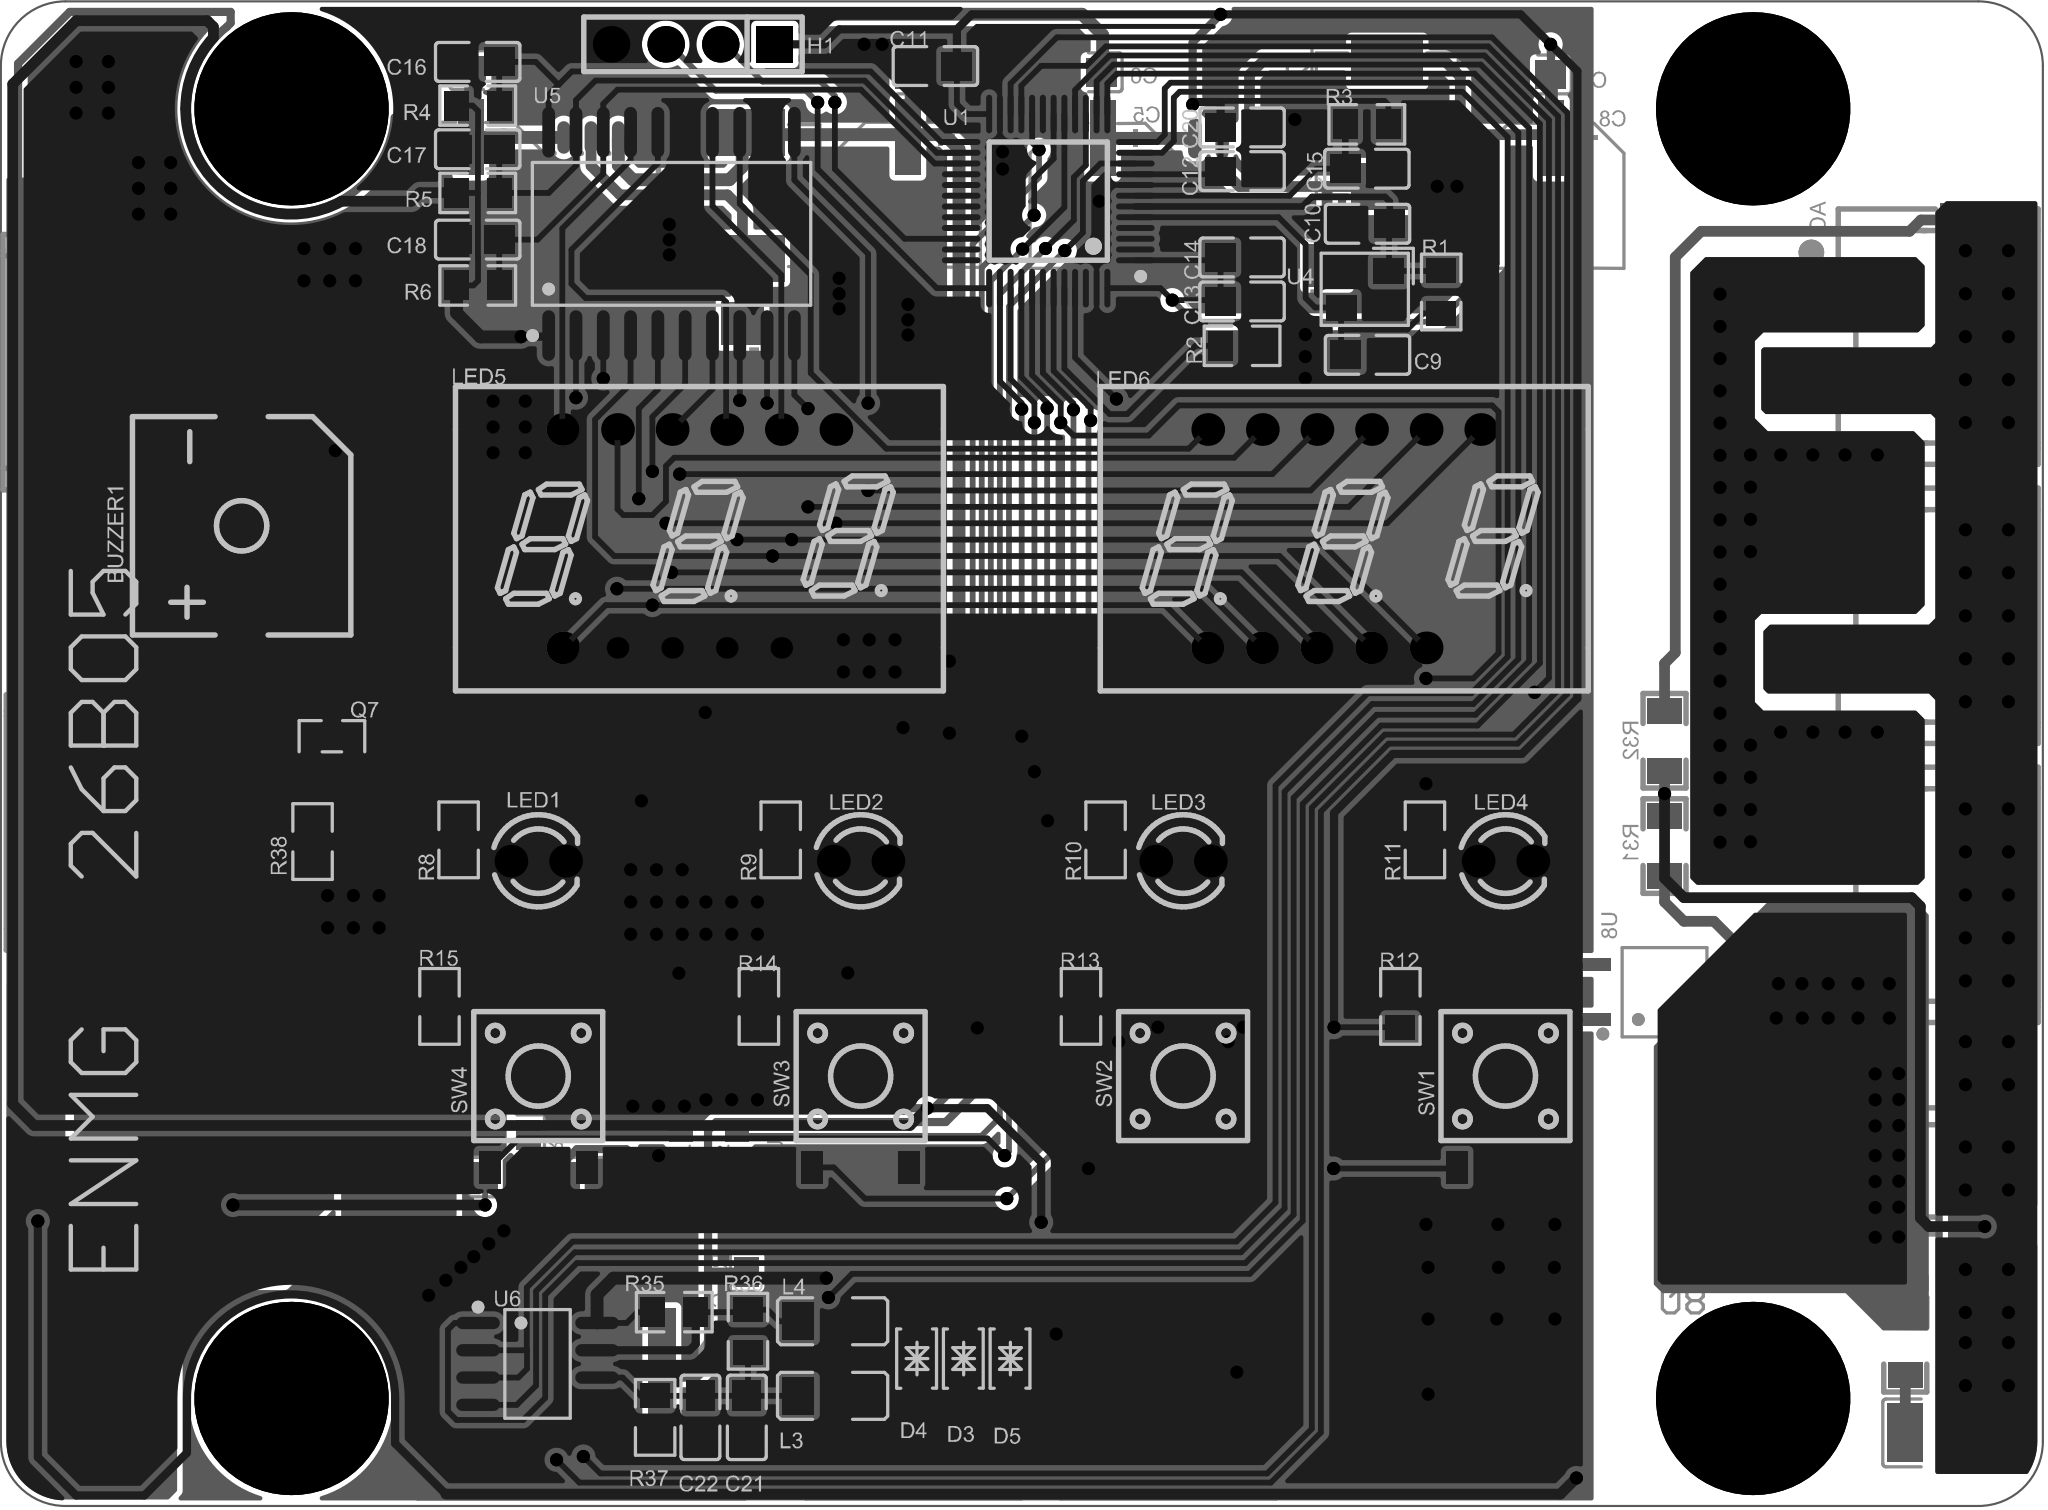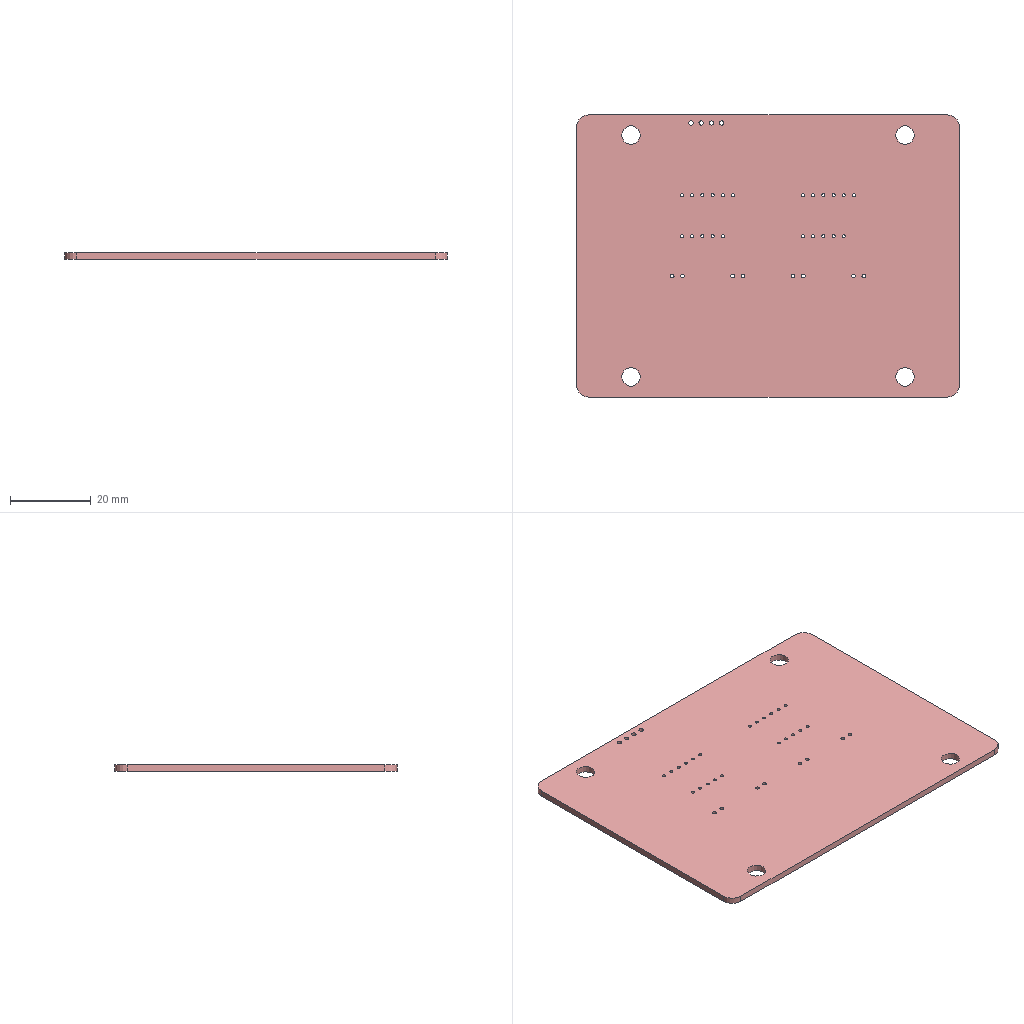Circuit board layout | Altium Designer | box 95 x 70 x 1.6 mm
Layer stack:
# Altium Designer layer stack of  (unit mm; dielectric type: 0 none, 1 core, 2 prepreg, 3 surface material)
index,name,kind,layer,copper_thickness_mm,dielectric_type,dielectric_thickness_mm,dielectric_material,dielectric_constant
0,Top Paste Mask Layer,other,,,,,,
1,Top Silkscreen Layer,other,,,,,,
2,Top Solder Mask Layer,dielectric,,,3,0.0102,,3.3
3,Top Layer,copper,Top Layer,0.0356,,,,
4,Dielectric1,dielectric,,,3,1.509,FR4,4.5
5,Bottom Layer,copper,Bottom Layer,0.0356,,,,
6,Bottom Solder Mask Layer,dielectric,,,3,0.0102,,3.3
7,Bottom Silkscreen Layer,other,,,,,,
8,Bottom Paste Mask Layer,other,,,,,,
# drill layer pairs: low layer,high layer
drill_pair,Top Layer,Bottom Layer
Part placement:
Designator,Comment,Layer,Footprint,Center-X(mm),Center-Y(mm),Rotation
C5,220uF,BottomLayer,CAP-SMD_BD6.3-L6.6-W6.6-FD,129.657,145.853,270
C4,220uF,BottomLayer,CAP-SMD_BD6.3-L6.6-W6.6-FD,120.594,145.898,270
C1,220uF,BottomLayer,CAP-SMD_BD6.3-L6.6-W6.6-FD,100.259,145.898,270
H1,PZ254V-11-04P,TopLayer,HDR-TH_4P-P2.54-V-M,110.599,152.9,180
C8,220uF,BottomLayer,CAP-SMD_BD6.3-L6.6-W6.6-FD,150.536,145.853,270
D1,SS34,BottomLayer,SMA_L4.3-W2.6-LS5.2-RD,110.701,139.901,180
D2,SS34,BottomLayer,SMA_L4.3-W2.6-LS5.2-RD,142.301,142.601,0
C23,10nF,BottomLayer,C1210,168.518,88.301,180
SW1,1TS005F-2500-5001,TopLayer,SW-SMD_4P-L6.0-W6.0-P4.50-LS9.0-H2.5,148.399,104.9,90
SW2,1TS005F-2500-5001,TopLayer,SW-SMD_4P-L6.0-W6.0-P4.50-LS9.0-H2.5,133.399,104.9,90
SW3,1TS005F-2500-5001,TopLayer,SW-SMD_4P-L6.0-W6.0-P4.50-LS9.0-H2.5,118.4,104.9,90
SW4,1TS005F-2500-5001,TopLayer,SW-SMD_4P-L6.0-W6.0-P4.50-LS9.0-H2.5,103.4,104.9,90
U1,GD32F103C8T6,TopLayer,TQFP-48_L7.0-W7.0-P0.50-LS9.0-BL,127.128,145.607,90
U2,XL1509-5.0,BottomLayer,SOIC-8_L4.9-W3.9-P1.27-LS6.0-TR,106.492,145.828,180
U3,XL1509-3.3E1,BottomLayer,SOP-8_L4.9-W3.9-P1.27-LS6.0-BL,135.854,145.84,0
LED1,3mmFIR,TopLayer,LED-TH_BD3.0-P2.54-FD,103.401,114.899,0
LED2,3mmFIR,TopLayer,LED-TH_BD3.0-P2.54-FD,118.4,114.899,0
LED3,3mmFIR,TopLayer,LED-TH_BD3.0-P2.54-FD,133.401,114.899,0
LED4,3mmFIR,TopLayer,LED-TH_BD3.0-P2.54-FD,148.399,114.899,0
U4,8MHz,TopLayer,CRYSTAL-SMD_4P-L3.2-W2.5-BL,141.854,141.505,180
U5,TM1620,TopLayer,SOIC-20_L13.0-W7.6-P1.27-LS10.3-BL,109.601,144.082,0
Q2,SS8050(RANGE:200-350),BottomLayer,SOT-23-3_L2.9-W1.3-P1.90-LS2.4-BR,119.733,106.553,90
Q3,SS8050(RANGE:200-350),BottomLayer,SOT-23-3_L2.9-W1.3-P1.90-LS2.4-BR,113.205,118.769,90
Q6,SS8050(RANGE:200-350),BottomLayer,SOT-23-3_L2.9-W1.3-P1.90-LS2.4-BR,149.02,110.03,180
R22,10K,BottomLayer,R0805,119.683,109.713,180
R26,10K,BottomLayer,R0805,113.156,121.816,180
R28,10K,BottomLayer,R0805,146.019,110.08,270
R29,10K,BottomLayer,R0805,147.02,107.201,180
R33,120Ω,BottomLayer,R0204,167,92.4,90
R31,51Ω,BottomLayer,R0204,155.801,115.6,90
R32,150Ω,BottomLayer,R0204,155.801,120.5,90
U8,ELM3083(TA)-V,BottomLayer,SOP-4_L4.4-W4.0-P2.54-LS7.0-TL,155.8,108.801,0
LED5,SP420361N,TopLayer,LED-SEG-TH_SP420361N,110.899,129.901,270
LED6,SP420361N,TopLayer,LED-SEG-TH_SP420361N,140.899,129.901,270
D3,SMF36CA,TopLayer,SOD-123_L2.7-W1.8-LS3.7-BI,123.177,91.757,90
D4,SMF36CA,TopLayer,SOD-123_L2.7-W1.8-LS3.7-BI,121.003,91.757,90
D5,SMF36CA,TopLayer,SOD-123_L2.7-W1.8-LS3.7-BI,125.349,91.757,90
U6,MAX485ESA(UMW),TopLayer,SOP-8_L5.0-W4.0-P1.27-LS6.0-BL,103.368,91.509,270
AC,VH3.96-2P 立贴,BottomLayer,CONN-SMD_2P-P3.96_HCTL_HC-VH-2ALT,167.132,139.3,270
AC1,VH3.96-2P 立贴,BottomLayer,CONN-SMD_2P-P3.96_HCTL_HC-VH-2ALT,167.132,126.314,270
C2,100nF,BottomLayer,C0805,101.258,151.699,0
C3,100nF,BottomLayer,C0805,119.7,151.501,0
C6,100nF,BottomLayer,C0805,128.6,151.6,180
C7,100nF,BottomLayer,C0805,149.501,151.501,0
C9,20pF,TopLayer,C0805,141.981,138.455,180
C10,20pF,TopLayer,C0805,141.981,144.551,0
C11,100nF,TopLayer,C0805,121.878,151.892,0
C12,100nF,TopLayer,C0805,136.145,147.002,180
C13,100nF,TopLayer,C0805,136.145,140.937,180
C14,100nF,TopLayer,C0805,136.145,142.987,180
C15,100nF,TopLayer,C0805,141.95,147.114,180
C16,100pF,TopLayer,C0805,100.585,152.083,0
C17,100pF,TopLayer,C0805,100.585,148.018,0
C18,100pF,TopLayer,C0805,100.585,143.815,0
C19,100nF,BottomLayer,C0805,114.101,93.701,0
C20,100nF,TopLayer,C0805,136.145,149.035,180
C21,100nF,TopLayer,C0805,113.104,89.023,90
C22,100nF,TopLayer,C0805,110.945,89.023,90
DC,VH3.96-2P 立贴,BottomLayer,CONN-SMD_2P-P3.96_HCTL_HC-VH-2ALT,84.55,138.113,90
HTR,VH3.96-2P 立贴,BottomLayer,CONN-SMD_2P-P3.96_HCTL_HC-VH-2ALT,167.132,113.33,270
Q1,NCE0140K2-VB,BottomLayer,TO-252-3_L6.6-W6.1-P4.58-LS10.1-BR,106.6,107.4,0
R12,4.7kΩ,TopLayer,R0805,143.51,108.141,270
R13,4.7kΩ,TopLayer,R0805,128.651,108.141,270
R14,4.7kΩ,TopLayer,R0805,113.665,108.141,270
R15,4.7kΩ,TopLayer,R0805,98.806,108.141,270
R8,100Ω,TopLayer,R0805,99.695,115.888,90
R9,100Ω,TopLayer,R0805,114.681,115.888,90
R10,100Ω,TopLayer,R0805,129.794,115.888,90
R11,100Ω,TopLayer,R0805,144.653,115.888,90
R27,10kΩ,BottomLayer,R0805,109.142,121.816,0
R17,1kΩ,BottomLayer,R0805,101.929,100.201,180
R18,1kΩ,BottomLayer,R0805,101.929,102.177,180
R25,4.7kΩ,BottomLayer,R0805,109.142,117.77,0
R21,1kΩ,BottomLayer,R0805,115.874,107.554,0
R1,1MΩ,TopLayer,R0805,145.41,141.378,270
R3,10kΩ,TopLayer,R0805,141.95,149.177,0
R2,10kΩ,TopLayer,R0805,136.145,138.875,180
R4,10kΩ,TopLayer,R0805,100.585,150.05,180
R5,10kΩ,TopLayer,R0805,100.585,145.987,180
R6,10kΩ,TopLayer,R0805,100.585,141.684,180
R7,10kΩ,BottomLayer,R0805,114.101,95.801,180
R20,4.7kΩ,BottomLayer,R0805,115.874,105.552,0
R24,1kΩ,BottomLayer,R0805,109.142,119.769,0
R23,10kΩ,BottomLayer,R0805,115.874,109.713,0
R16,24kΩ,BottomLayer,R0805,105.739,100.201,0
U7,LMV321,BottomLayer,SOT-23-5_L3.0-W1.7-P0.95-LS2.8-BR,111.347,101.168,180
R30,10K,BottomLayer,R0805,147.02,104.699,180
R35,47kΩ,TopLayer,R0805,109.729,93.916,180
R36,12kΩ,TopLayer,R0805,113.157,93.028,90
R37,47kΩ,TopLayer,R0805,108.839,89.023,90
485,XH2.54-2P立贴,BottomLayer,CONN-SMD_2P_A2501WV-S,132.78,89.346,180
AD,XH2.54-2P立贴,BottomLayer,CONN-SMD_2P_A2501WV-S,120.928,89.346,180
Q4,HYG025N06LS1B,BottomLayer,TO-263-2_L10.2-W8.7-P5.08-LS15.1-BR,96.5,130.801,90
TEC,VH3.96-2P 立贴,BottomLayer,CONN-SMD_2P-P3.96_HCTL_HC-VH-2ALT,84.7,116.7,90
FAN,XH2.54-2P立贴,BottomLayer,CONN-SMD_2P_A2501WV-S,82.864,104.068,90
FAN2,XH2.54-2P立贴,BottomLayer,CONN-SMD_2P_A2501WV-S,94,104.068,90
L3,22uH,TopLayer,L1206,117.094,90.023,0
L4,22uH,TopLayer,L1206,117.094,93.492,0
R19,10mΩ,BottomLayer,R2010,92.6,96.799,180
BUZZER1,2.7kHz,TopLayer,BUZ-SMD_L9.6-W9.6-LS10.0-R,89.601,130.5,270
Q7,SS8050(RANGE:200-350),TopLayer,SOT-23-3_L2.9-W1.3-P1.90-LS2.4-BR,93.802,120.711,270
R38,1kΩ,TopLayer,R0805,92.9,115.81,90
TH,HX 2.54-4P LT,BottomLayer,CONN-SMD_4P-P2.50_HX-2.54-4P-LT,105.4,89.046,180
Q8,BTA216B-600D-JSM,BottomLayer,TO-263-3_L10.2-W9.2-P5.08-LS15.4-BR,165.5,100.5,0
L1,68uH,BottomLayer,IND-SMD_L7.1-W6.6_H5.0,113.2,145.862,270
L2,68uH,BottomLayer,IND-SMD_L7.1-W6.6_H5.0,142.9,149.2,270
Pad and via stacks:
# Altium Designer via and pad stacks of  (unit mm). Each distinct definition once, with the count of objects using it.
# via: kind,start_layer,end_layer,hole_mm,diameter_mm,mode(0 simple;1 top-mid-bottom;2 full stack),diameter_per_layer,count,example_net
# pad: kind,layer,hole_mm,hole_type(0 round;1 square;2 slot),plating,top_size,top_shape(1 round;2 rect;3 octagon;9 rounded rect),mid_size,bottom_size,mode,footprint,size_per_layer,count,example
pad,Multi-Layer,4.6,0,plated,8.999x8.999,1,5.001x5.001,8.999x8.999,1,,,4,1
pad,Multi-Layer,1.1,0,plated,1.699x1.699,2,1.699x1.699,1.699x1.699,0,HDR-TH_4P-P2.54-V-M,,1,H1.1
pad,Multi-Layer,1.1,0,plated,1.699x1.699,1,1.699x1.699,1.699x1.699,0,HDR-TH_4P-P2.54-V-M,,3,H1.2
pad,Multi-Layer,0.9144,0,plated,1.524x1.524,1,1.524x1.524,1.524x1.524,0,LED-TH_BD3.0-P2.54-FD,,8,LED1.1
pad,Multi-Layer,0.762,0,plated,1.001x1.001,1,1.001x1.001,1.524x1.524,1,LED-SEG-TH_SP420361N,,22,LED5.1
pad,Bottom Layer,0,0,plated,3.5x1.199,2,3.5x1.199,3.5x1.199,0,CAP-SMD_BD6.3-L6.6-W6.6-FD,,8,C5.1
pad,Bottom Layer,0,0,plated,1.999x1.999,2,1.999x1.999,1.999x1.999,0,SMA_L4.3-W2.6-LS5.2-RD,,4,D1.2
pad,Bottom Layer,0,0,plated,1.636x2.7,2,1.636x2.7,1.636x2.7,0,C1210,,2,C23.2
pad,Bottom Layer,0,0,plated,0.5994x1.519,1,0.5994x1.519,0.5994x1.519,0,SOIC-8_L4.9-W3.9-P1.27-LS6.0-TR,,8,U2.5
pad,Bottom Layer,0,0,plated,0.6299x1.864,1,0.6299x1.864,0.6299x1.864,0,SOP-8_L4.9-W3.9-P1.27-LS6.0-BL,,8,U3.1
pad,Bottom Layer,0,0,plated,1.25x0.701,2,1.25x0.701,1.25x0.701,0,SOT-23-3_L2.9-W1.3-P1.90-LS2.4-BR,,9,Q2.1
pad,Bottom Layer,0,0,plated,1.133x1.377,2,1.133x1.377,1.133x1.377,0,R0805,,30,R22.2
pad,Bottom Layer,0,0,plated,1.199x1.6,2,1.199x1.6,1.199x1.6,0,R0204,,6,R33.2
pad,Bottom Layer,0,0,plated,0.5944x1.3,2,0.5944x1.3,0.5944x1.3,0,SOP-4_L4.4-W4.0-P2.54-LS7.0-TL,,4,U8.1
pad,Bottom Layer,0,0,plated,2.499x7,2,2.499x7,2.499x7,0,CONN-SMD_2P-P3.96_HCTL_HC-VH-2ALT,,10,AC.1
pad,Bottom Layer,0,0,plated,1.501x3,2,1.501x3,1.501x3,0,CONN-SMD_2P-P3.96_HCTL_HC-VH-2ALT,,10,AC.3
pad,Bottom Layer,0,0,plated,1.41x1.349,2,1.41x1.349,1.41x1.349,0,C0805,,10,C2.2
pad,Bottom Layer,0,0,plated,6.5x6,2,6.5x6,6.5x6,0,TO-252-3_L6.6-W6.1-P4.58-LS10.1-BR,,1,Q1.3
pad,Bottom Layer,0,0,plated,3x1.6,2,3x1.6,3x1.6,0,TO-252-3_L6.6-W6.1-P4.58-LS10.1-BR,,2,Q1.1
pad,Bottom Layer,0,0,plated,1.1x0.5994,2,1.1x0.5994,1.1x0.5994,0,SOT-23-5_L3.0-W1.7-P0.95-LS2.8-BR,,5,U7.5
pad,Bottom Layer,0,0,plated,1.1x2.499,2,1.1x2.499,1.1x2.499,0,CONN-SMD_2P_A2501WV-S,,8,485.4
pad,Bottom Layer,0,0,plated,1.199x5.7,2,1.199x5.7,1.199x5.7,0,CONN-SMD_2P_A2501WV-S,,8,485.1
pad,Bottom Layer,0,0,plated,8.839x11.001,2,8.839x11.001,8.839x11.001,0,TO-263-2_L10.2-W8.7-P5.08-LS15.1-BR,,1,Q4.4
pad,Bottom Layer,0,0,plated,3.81x1.999,2,3.81x1.999,3.81x1.999,0,TO-263-2_L10.2-W8.7-P5.08-LS15.1-BR,,2,Q4.3
pad,Bottom Layer,0,0,plated,1.283x2.7,2,1.283x2.7,1.283x2.7,0,R2010,,2,R19.2
pad,Bottom Layer,0,0,plated,1.3x6.5,2,1.3x6.5,1.3x6.5,0,CONN-SMD_4P-P2.50_HX-2.54-4P-LT,,4,TH.4
pad,Bottom Layer,0,0,plated,1.801x3,2,1.801x3,1.801x3,0,CONN-SMD_4P-P2.50_HX-2.54-4P-LT,,2,TH.6
pad,Bottom Layer,0,0,plated,3.8x1.399,2,3.8x1.399,3.8x1.399,0,TO-263-3_L10.2-W9.2-P5.08-LS15.4-BR,,2,Q8.1
pad,Bottom Layer,0,0,plated,8.801x10.701,2,8.801x10.701,8.801x10.701,0,TO-263-3_L10.2-W9.2-P5.08-LS15.4-BR,,1,Q8.2
pad,Bottom Layer,0,0,plated,2.149x3.32,2,2.149x3.32,2.149x3.32,0,IND-SMD_L7.1-W6.6_H5.0,,4,L1.2
pad,Top Layer,0,0,plated,1.501x1.001,2,1.501x1.001,1.501x1.001,0,SW-SMD_4P-L6.0-W6.0-P4.50-LS9.0-H2.5,,16,SW1.1
pad,Top Layer,0,0,plated,0.2794x1.801,1,0.2794x1.801,0.2794x1.801,0,TQFP-48_L7.0-W7.0-P0.50-LS9.0-BL,,24,U1.1
pad,Top Layer,0,0,plated,1.801x0.2794,1,1.801x0.2794,1.801x0.2794,0,TQFP-48_L7.0-W7.0-P0.50-LS9.0-BL,,24,U1.13
pad,Top Layer,0,0,plated,1.399x1.199,2,1.399x1.199,1.399x1.199,0,CRYSTAL-SMD_4P-L3.2-W2.5-BL,,4,U4.1
pad,Top Layer,0,0,plated,0.5944x2.36,1,0.5944x2.36,0.5944x2.36,0,SOIC-20_L13.0-W7.6-P1.27-LS10.3-BL,,20,U5.1
pad,Top Layer,0,0,plated,1.399x1.199,2,1.399x1.199,1.399x1.199,0,SOD-123_L2.7-W1.8-LS3.7-BI,,6,D3.2
pad,Top Layer,0,0,plated,0.574x2.034,1,0.574x2.034,0.574x2.034,0,SOP-8_L5.0-W4.0-P1.27-LS6.0-BL,,8,U6.1
pad,Top Layer,0,0,plated,1.41x1.349,2,1.41x1.349,1.41x1.349,0,C0805,,26,C9.2
pad,Top Layer,0,0,plated,1.133x1.377,2,1.133x1.377,1.133x1.377,0,R0805,,36,R12.2
pad,Top Layer,0,0,plated,1.486x1.727,2,1.486x1.727,1.486x1.727,0,L1206,,4,L3.2
pad,Top Layer,0,0,plated,2.499x1.801,2,2.499x1.801,2.499x1.801,0,BUZ-SMD_L9.6-W9.6-LS10.0-R,,2,BUZZER1.1
pad,Top Layer,0,0,plated,1.25x0.701,2,1.25x0.701,1.25x0.701,0,SOT-23-3_L2.9-W1.3-P1.90-LS2.4-BR,,3,Q7.1
via,Top Layer,Bottom Layer,0.3048,0.6096,0,,334,6
Copper pours:
name,layer,net,type(0 solid;1 hatched;2 none)
Top Layer-GND,Top Layer,GND,0
Top Layer-N,Top Layer,N,0
Top Layer-L,Top Layer,L,0
Top Layer-HTR1,Top Layer,HTR1,0
Bottom Layer-VCC,Bottom Layer,VCC,0
Bottom Layer-PL,Bottom Layer,PL,0
Bottom Layer-FAN1,Bottom Layer,FAN1,0
Bottom Layer-FAN2,Bottom Layer,FAN2,0
Bottom Layer-GND,Bottom Layer,GND,0
Bottom Layer-N,Bottom Layer,N,0
Bottom Layer-L,Bottom Layer,L,0
Bottom Layer-HTR1,Bottom Layer,HTR1,0
Design rules, without the lines most boards share:
# Altium Designer design rules of  (exported by Altium Designer, unit mm)
# columns: name | kind | enabled | priority | scope1 | scope2 | descriptor | typed fields (field=value)
HoleToHoleClearance | 52 | enabled | 1 | All | All | Hole To Hole Clearance (Gap=10mil) (All),(All) | gap=0.254
copperThickness1oz | 0 | enabled | 2 | All | All | Clearance Constraint (Gap=7mil) (All),(All) | gap=0.1778
copperThickness2oz | 0 | enabled | 1 | All | All | Clearance Constraint (Gap=7mil) (All),(All) | gap=0.1778
copperThickness2oz_1 | 63 | enabled | 1 | All | All | Board Clearance Constraint (Gap=0mil) (All) |
Plane_innerPlane | 0 | enabled | 3 | All | All | Clearance Constraint (Gap=7mil) (All),(All) | gap=0.1778
Plane_innerPlane_1 | 63 | enabled | 3 | All | All | Board Clearance Constraint (Gap=0mil) (All) |
Copper_copperRegion | 0 | enabled | 5 | All | All | Clearance Constraint (Gap=7mil) (All),(All) | gap=0.1778
Copper_copperRegion_1 | 63 | enabled | 5 | All | All | Board Clearance Constraint (Gap=0mil) (All) |
otherClearance | 0 | enabled | 4 | All | All | Clearance Constraint (Gap=7mil) (All),(All) | gap=0.1778
otherClearance_1 | 63 | enabled | 4 | All | All | Board Clearance Constraint (Gap=0mil) (All) |
copperThickness1oz_2 | 2 | enabled | 1 | All | All | Width Constraint (Min=5mil) (Max=100mil) (Preferred=10mil) (All) |
copperThickness2oz_2 | 2 | enabled | 2 | All | All | Width Constraint (Min=8mil) (Max=100mil) (Preferred=10mil) (All) |
trackWidth1 | 2 | enabled | 3 | All | All | Width Constraint (Min=5mil) (Max=100mil) (Preferred=30mil) (All) |
viaSize | 11 | enabled | 1 | All | All | Routing Via (MinHoleWidth=11.811mil) (MaxHoleWidth=248.031mil) (PreferredHoleWidth=12.008mil) (MinWidth=11.811mil) (MaxWidth=248.031mil) (PreferedWidth=12.008mil) (All) | via_min_hole=0.3 via_max_hole=6.3 via_preferred_diameter=0.305 via_preferred_hole=0.305
copperRegion | 20 | enabled | 1 | All | All | Polygon Connect Rule(Direct Connect )(Conductor Width=10mil) (Relief Angle=90 Angle) (Entries=4) (Air Gap Width=10mil) (All),(All) | connect_style(0=relief,1=direct,2=none)=1 relief_conductor_width=0.254 relief_entries=4